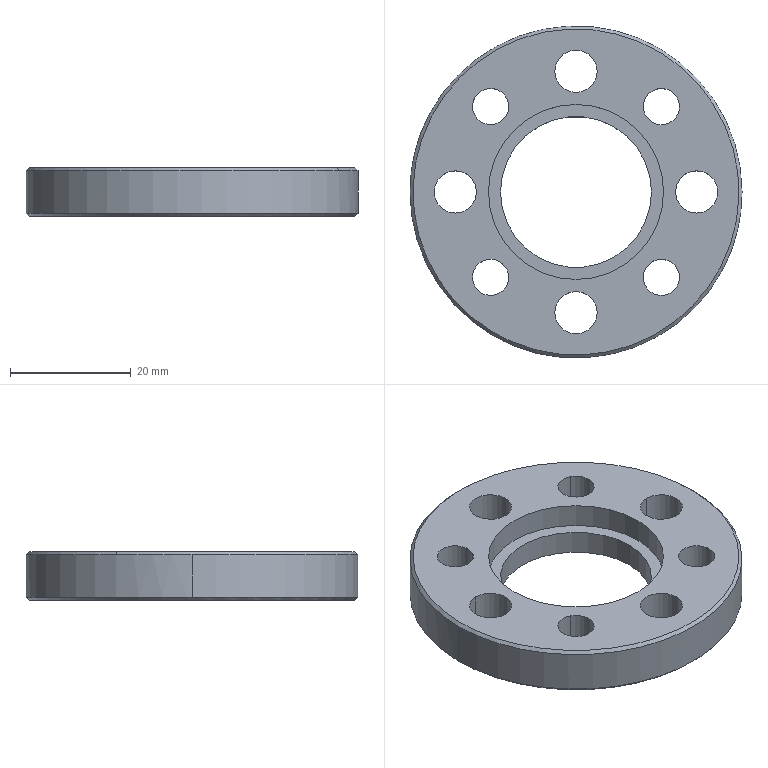Part | STEP file | Flange.1.stp | 1 solid | 29 faces | box 55 x 55 x 8 mm | volume 12222 mm3 | cylinder 22 | cone 4 | plane 3 | commonest cylinder face diameters 6 x8 7 x8 25 x2 29 x2 55 x2